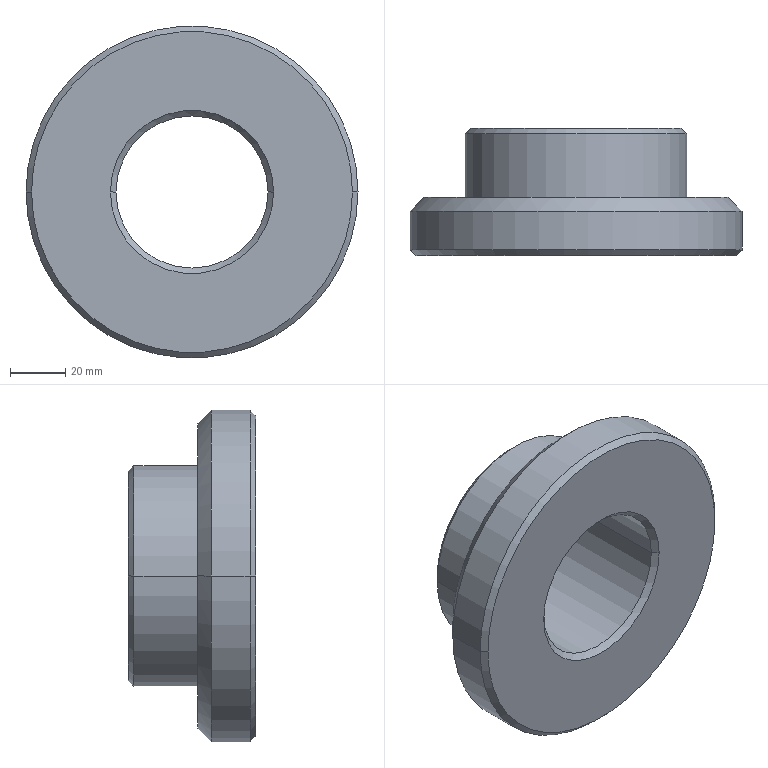Part | SolidWorks | features Revolution 1 | 1 solid | 19 faces | box 120 x 46 x 120 mm | volume 247351 mm3 | cone 10 | cylinder 6 | plane 3 | commonest cylinder face diameters 55 x2 80 x2 120 x2
STEP:
#1=CARTESIAN_POINT('',(-55.,21.,0.));
#2=VERTEX_POINT('',#1);
#3=CARTESIAN_POINT('',(55.,21.,0.));
#4=VERTEX_POINT('',#3);
#5=CARTESIAN_POINT('',(0.,21.,0.));
#6=DIRECTION('',(0.,1.,0.));
#7=DIRECTION('',(-1.,0.,0.));
#8=AXIS2_PLACEMENT_3D('',#5,#6,#7);
#9=CIRCLE('',#8,55.);
#10=EDGE_CURVE('',#2,#4,#9,.T.);
#11=ORIENTED_EDGE('',*,*,#10,.F.);
#12=CARTESIAN_POINT('',(-60.,16.,0.));
#13=VERTEX_POINT('',#12);
#14=CARTESIAN_POINT('',(-55.,21.,0.));
#15=DIRECTION('',(-0.7071,-0.7071,0.));
#16=VECTOR('',#15,1000.);
#17=LINE('',#14,#16);
#18=EDGE_CURVE('',#2,#13,#17,.T.);
#19=ORIENTED_EDGE('',*,*,#18,.T.);
#20=CARTESIAN_POINT('',(60.,16.,0.));
#21=VERTEX_POINT('',#20);
#22=CARTESIAN_POINT('',(0.,16.,0.));
#23=DIRECTION('',(0.,1.,0.));
#24=DIRECTION('',(-1.,0.,0.));
#25=AXIS2_PLACEMENT_3D('',#22,#23,#24);
#26=CIRCLE('',#25,60.);
#27=EDGE_CURVE('',#13,#21,#26,.T.);
#28=ORIENTED_EDGE('',*,*,#27,.T.);
#29=CARTESIAN_POINT('',(55.,21.,0.));
#30=DIRECTION('',(0.7071,-0.7071,0.));
#31=VECTOR('',#30,1000.);
#32=LINE('',#29,#31);
#33=EDGE_CURVE('',#4,#21,#32,.T.);
#34=ORIENTED_EDGE('',*,*,#33,.F.);
#35=EDGE_LOOP('',(#11,#19,#28,#34));
#36=FACE_OUTER_BOUND('',#35,.T.);
#37=CARTESIAN_POINT('',(0.,21.,0.));
#38=DIRECTION('',(0.,-1.,0.));
#39=DIRECTION('',(1.,0.,0.));
#40=AXIS2_PLACEMENT_3D('',#37,#38,#39);
#41=CONICAL_SURFACE('',#40,55.,0.7854);
#42=ADVANCED_FACE('',(#36),#41,.T.);
#43=CARTESIAN_POINT('',(-60.,2.,0.));
#44=VERTEX_POINT('',#43);
#45=CARTESIAN_POINT('',(60.,2.,0.));
#46=VERTEX_POINT('',#45);
#47=CARTESIAN_POINT('',(0.,2.,0.));
#48=DIRECTION('',(0.,1.,0.));
#49=DIRECTION('',(-1.,0.,0.));
#50=AXIS2_PLACEMENT_3D('',#47,#48,#49);
#51=CIRCLE('',#50,60.);
#52=EDGE_CURVE('',#44,#46,#51,.T.);
#53=ORIENTED_EDGE('',*,*,#52,.T.);
#54=CARTESIAN_POINT('',(60.,46.,0.));
#55=DIRECTION('',(0.,1.,0.));
#56=VECTOR('',#55,1000.);
#57=LINE('',#54,#56);
#58=EDGE_CURVE('',#46,#21,#57,.T.);
#59=ORIENTED_EDGE('',*,*,#58,.T.);
#60=ORIENTED_EDGE('',*,*,#27,.F.);
#61=CARTESIAN_POINT('',(-60.,46.,0.));
#62=DIRECTION('',(0.,1.,0.));
#63=VECTOR('',#62,1000.);
#64=LINE('',#61,#63);
#65=EDGE_CURVE('',#44,#13,#64,.T.);
#66=ORIENTED_EDGE('',*,*,#65,.F.);
#67=EDGE_LOOP('',(#53,#59,#60,#66));
#68=FACE_OUTER_BOUND('',#67,.T.);
#69=CARTESIAN_POINT('',(0.,46.,0.));
#70=DIRECTION('',(0.,1.,0.));
#71=DIRECTION('',(-1.,0.,0.));
#72=AXIS2_PLACEMENT_3D('',#69,#70,#71);
#73=CYLINDRICAL_SURFACE('',#72,60.);
#74=ADVANCED_FACE('',(#68),#73,.T.);
#75=CARTESIAN_POINT('',(-58.,0.,0.));
#76=VERTEX_POINT('',#75);
#77=CARTESIAN_POINT('',(58.,0.,0.));
#78=VERTEX_POINT('',#77);
#79=CARTESIAN_POINT('',(0.,0.,0.));
#80=DIRECTION('',(0.,1.,0.));
#81=DIRECTION('',(-1.,0.,0.));
#82=AXIS2_PLACEMENT_3D('',#79,#80,#81);
#83=CIRCLE('',#82,58.);
#84=EDGE_CURVE('',#76,#78,#83,.T.);
#85=ORIENTED_EDGE('',*,*,#84,.T.);
#86=CARTESIAN_POINT('',(60.,2.,0.));
#87=DIRECTION('',(0.7071,0.7071,0.));
#88=VECTOR('',#87,1000.);
#89=LINE('',#86,#88);
#90=EDGE_CURVE('',#78,#46,#89,.T.);
#91=ORIENTED_EDGE('',*,*,#90,.T.);
#92=ORIENTED_EDGE('',*,*,#52,.F.);
#93=CARTESIAN_POINT('',(-60.,2.,0.));
#94=DIRECTION('',(-0.7071,0.7071,0.));
#95=VECTOR('',#94,1000.);
#96=LINE('',#93,#95);
#97=EDGE_CURVE('',#76,#44,#96,.T.);
#98=ORIENTED_EDGE('',*,*,#97,.F.);
#99=EDGE_LOOP('',(#85,#91,#92,#98));
#100=FACE_OUTER_BOUND('',#99,.T.);
#101=CARTESIAN_POINT('',(0.,2.,0.));
#102=DIRECTION('',(0.,1.,0.));
#103=DIRECTION('',(-1.,0.,0.));
#104=AXIS2_PLACEMENT_3D('',#101,#102,#103);
#105=CONICAL_SURFACE('',#104,60.,0.7854);
#106=ADVANCED_FACE('',(#100),#105,.T.);
#107=CARTESIAN_POINT('',(27.5,2.,0.));
#108=VERTEX_POINT('',#107);
#109=CARTESIAN_POINT('',(-27.5,2.,0.));
#110=VERTEX_POINT('',#109);
#111=CARTESIAN_POINT('',(0.,2.,0.));
#112=DIRECTION('',(0.,1.,0.));
#113=DIRECTION('',(-1.,0.,0.));
#114=AXIS2_PLACEMENT_3D('',#111,#112,#113);
#115=CIRCLE('',#114,27.5);
#116=EDGE_CURVE('',#108,#110,#115,.T.);
#117=ORIENTED_EDGE('',*,*,#116,.T.);
#118=CARTESIAN_POINT('',(-29.5,0.,0.));
#119=VERTEX_POINT('',#118);
#120=CARTESIAN_POINT('',(-29.5,0.,0.));
#121=DIRECTION('',(-0.7071,-0.7071,0.));
#122=VECTOR('',#121,1000.);
#123=LINE('',#120,#122);
#124=EDGE_CURVE('',#110,#119,#123,.T.);
#125=ORIENTED_EDGE('',*,*,#124,.T.);
#126=CARTESIAN_POINT('',(29.5,0.,0.));
#127=VERTEX_POINT('',#126);
#128=CARTESIAN_POINT('',(0.,0.,0.));
#129=DIRECTION('',(0.,1.,0.));
#130=DIRECTION('',(-1.,0.,0.));
#131=AXIS2_PLACEMENT_3D('',#128,#129,#130);
#132=CIRCLE('',#131,29.5);
#133=EDGE_CURVE('',#127,#119,#132,.T.);
#134=ORIENTED_EDGE('',*,*,#133,.F.);
#135=CARTESIAN_POINT('',(29.5,0.,0.));
#136=DIRECTION('',(0.7071,-0.7071,0.));
#137=VECTOR('',#136,1000.);
#138=LINE('',#135,#137);
#139=EDGE_CURVE('',#108,#127,#138,.T.);
#140=ORIENTED_EDGE('',*,*,#139,.F.);
#141=EDGE_LOOP('',(#117,#125,#134,#140));
#142=FACE_OUTER_BOUND('',#141,.T.);
#143=CARTESIAN_POINT('',(0.,0.,0.));
#144=DIRECTION('',(0.,-1.,0.));
#145=DIRECTION('',(1.,0.,0.));
#146=AXIS2_PLACEMENT_3D('',#143,#144,#145);
#147=CONICAL_SURFACE('',#146,29.5,0.7854);
#148=ADVANCED_FACE('',(#142),#147,.F.);
#149=ORIENTED_EDGE('',*,*,#116,.F.);
#150=CARTESIAN_POINT('',(27.5,44.,0.));
#151=VERTEX_POINT('',#150);
#152=CARTESIAN_POINT('',(27.5,46.,0.));
#153=DIRECTION('',(0.,1.,0.));
#154=VECTOR('',#153,1000.);
#155=LINE('',#152,#154);
#156=EDGE_CURVE('',#108,#151,#155,.T.);
#157=ORIENTED_EDGE('',*,*,#156,.T.);
#158=CARTESIAN_POINT('',(-27.5,44.,0.));
#159=VERTEX_POINT('',#158);
#160=CARTESIAN_POINT('',(0.,44.,0.));
#161=DIRECTION('',(0.,1.,0.));
#162=DIRECTION('',(-1.,0.,0.));
#163=AXIS2_PLACEMENT_3D('',#160,#161,#162);
#164=CIRCLE('',#163,27.5);
#165=EDGE_CURVE('',#151,#159,#164,.T.);
#166=ORIENTED_EDGE('',*,*,#165,.T.);
#167=CARTESIAN_POINT('',(-27.5,46.,0.));
#168=DIRECTION('',(0.,1.,0.));
#169=VECTOR('',#168,1000.);
#170=LINE('',#167,#169);
#171=EDGE_CURVE('',#110,#159,#170,.T.);
#172=ORIENTED_EDGE('',*,*,#171,.F.);
#173=EDGE_LOOP('',(#149,#157,#166,#172));
#174=FACE_OUTER_BOUND('',#173,.T.);
#175=CARTESIAN_POINT('',(0.,46.,0.));
#176=DIRECTION('',(0.,1.,0.));
#177=DIRECTION('',(-1.,0.,0.));
#178=AXIS2_PLACEMENT_3D('',#175,#176,#177);
#179=CYLINDRICAL_SURFACE('',#178,27.5);
#180=ADVANCED_FACE('',(#174),#179,.F.);
#181=ORIENTED_EDGE('',*,*,#165,.F.);
#182=CARTESIAN_POINT('',(29.5,46.,0.));
#183=VERTEX_POINT('',#182);
#184=CARTESIAN_POINT('',(27.5,44.,0.));
#185=DIRECTION('',(0.7071,0.7071,0.));
#186=VECTOR('',#185,1000.);
#187=LINE('',#184,#186);
#188=EDGE_CURVE('',#151,#183,#187,.T.);
#189=ORIENTED_EDGE('',*,*,#188,.T.);
#190=CARTESIAN_POINT('',(-29.5,46.,0.));
#191=VERTEX_POINT('',#190);
#192=CARTESIAN_POINT('',(0.,46.,0.));
#193=DIRECTION('',(0.,1.,0.));
#194=DIRECTION('',(-1.,0.,0.));
#195=AXIS2_PLACEMENT_3D('',#192,#193,#194);
#196=CIRCLE('',#195,29.5);
#197=EDGE_CURVE('',#183,#191,#196,.T.);
#198=ORIENTED_EDGE('',*,*,#197,.T.);
#199=CARTESIAN_POINT('',(-27.5,44.,0.));
#200=DIRECTION('',(-0.7071,0.7071,0.));
#201=VECTOR('',#200,1000.);
#202=LINE('',#199,#201);
#203=EDGE_CURVE('',#159,#191,#202,.T.);
#204=ORIENTED_EDGE('',*,*,#203,.F.);
#205=EDGE_LOOP('',(#181,#189,#198,#204));
#206=FACE_OUTER_BOUND('',#205,.T.);
#207=CARTESIAN_POINT('',(0.,44.,0.));
#208=DIRECTION('',(0.,1.,0.));
#209=DIRECTION('',(-1.,0.,0.));
#210=AXIS2_PLACEMENT_3D('',#207,#208,#209);
#211=CONICAL_SURFACE('',#210,27.5,0.7854);
#212=ADVANCED_FACE('',(#206),#211,.F.);
#213=CARTESIAN_POINT('',(-38.,46.,0.));
#214=VERTEX_POINT('',#213);
#215=CARTESIAN_POINT('',(38.,46.,0.));
#216=VERTEX_POINT('',#215);
#217=CARTESIAN_POINT('',(0.,46.,0.));
#218=DIRECTION('',(0.,1.,0.));
#219=DIRECTION('',(-1.,0.,0.));
#220=AXIS2_PLACEMENT_3D('',#217,#218,#219);
#221=CIRCLE('',#220,38.);
#222=EDGE_CURVE('',#214,#216,#221,.T.);
#223=ORIENTED_EDGE('',*,*,#222,.F.);
#224=CARTESIAN_POINT('',(-40.,44.,0.));
#225=VERTEX_POINT('',#224);
#226=CARTESIAN_POINT('',(-38.,46.,0.));
#227=DIRECTION('',(-0.7071,-0.7071,0.));
#228=VECTOR('',#227,1000.);
#229=LINE('',#226,#228);
#230=EDGE_CURVE('',#214,#225,#229,.T.);
#231=ORIENTED_EDGE('',*,*,#230,.T.);
#232=CARTESIAN_POINT('',(40.,44.,0.));
#233=VERTEX_POINT('',#232);
#234=CARTESIAN_POINT('',(0.,44.,0.));
#235=DIRECTION('',(0.,1.,0.));
#236=DIRECTION('',(-1.,0.,0.));
#237=AXIS2_PLACEMENT_3D('',#234,#235,#236);
#238=CIRCLE('',#237,40.);
#239=EDGE_CURVE('',#225,#233,#238,.T.);
#240=ORIENTED_EDGE('',*,*,#239,.T.);
#241=CARTESIAN_POINT('',(38.,46.,0.));
#242=DIRECTION('',(0.7071,-0.7071,0.));
#243=VECTOR('',#242,1000.);
#244=LINE('',#241,#243);
#245=EDGE_CURVE('',#216,#233,#244,.T.);
#246=ORIENTED_EDGE('',*,*,#245,.F.);
#247=EDGE_LOOP('',(#223,#231,#240,#246));
#248=FACE_OUTER_BOUND('',#247,.T.);
#249=CARTESIAN_POINT('',(0.,46.,0.));
#250=DIRECTION('',(0.,-1.,0.));
#251=DIRECTION('',(1.,0.,0.));
#252=AXIS2_PLACEMENT_3D('',#249,#250,#251);
#253=CONICAL_SURFACE('',#252,38.,0.7854);
#254=ADVANCED_FACE('',(#248),#253,.T.);
#255=CARTESIAN_POINT('',(-40.,21.,0.));
#256=VERTEX_POINT('',#255);
#257=CARTESIAN_POINT('',(40.,21.,0.));
#258=VERTEX_POINT('',#257);
#259=CARTESIAN_POINT('',(0.,21.,0.));
#260=DIRECTION('',(0.,1.,0.));
#261=DIRECTION('',(-1.,0.,0.));
#262=AXIS2_PLACEMENT_3D('',#259,#260,#261);
#263=CIRCLE('',#262,40.);
#264=EDGE_CURVE('',#256,#258,#263,.T.);
#265=ORIENTED_EDGE('',*,*,#264,.T.);
#266=CARTESIAN_POINT('',(40.,46.,0.));
#267=DIRECTION('',(0.,1.,0.));
#268=VECTOR('',#267,1000.);
#269=LINE('',#266,#268);
#270=EDGE_CURVE('',#258,#233,#269,.T.);
#271=ORIENTED_EDGE('',*,*,#270,.T.);
#272=ORIENTED_EDGE('',*,*,#239,.F.);
#273=CARTESIAN_POINT('',(-40.,46.,0.));
#274=DIRECTION('',(0.,1.,0.));
#275=VECTOR('',#274,1000.);
#276=LINE('',#273,#275);
#277=EDGE_CURVE('',#256,#225,#276,.T.);
#278=ORIENTED_EDGE('',*,*,#277,.F.);
#279=EDGE_LOOP('',(#265,#271,#272,#278));
#280=FACE_OUTER_BOUND('',#279,.T.);
#281=CARTESIAN_POINT('',(0.,46.,0.));
#282=DIRECTION('',(0.,1.,0.));
#283=DIRECTION('',(-1.,0.,0.));
#284=AXIS2_PLACEMENT_3D('',#281,#282,#283);
#285=CYLINDRICAL_SURFACE('',#284,40.);
#286=ADVANCED_FACE('',(#280),#285,.T.);
#287=ORIENTED_EDGE('',*,*,#270,.F.);
#288=CARTESIAN_POINT('',(0.,21.,0.));
#289=DIRECTION('',(0.,1.,0.));
#290=DIRECTION('',(-1.,0.,0.));
#291=AXIS2_PLACEMENT_3D('',#288,#289,#290);
#292=CIRCLE('',#291,40.);
#293=EDGE_CURVE('',#258,#256,#292,.T.);
#294=ORIENTED_EDGE('',*,*,#293,.T.);
#295=ORIENTED_EDGE('',*,*,#277,.T.);
#296=CARTESIAN_POINT('',(0.,44.,0.));
#297=DIRECTION('',(0.,1.,0.));
#298=DIRECTION('',(-1.,0.,0.));
#299=AXIS2_PLACEMENT_3D('',#296,#297,#298);
#300=CIRCLE('',#299,40.);
#301=EDGE_CURVE('',#233,#225,#300,.T.);
#302=ORIENTED_EDGE('',*,*,#301,.F.);
#303=EDGE_LOOP('',(#287,#294,#295,#302));
#304=FACE_OUTER_BOUND('',#303,.T.);
#305=CARTESIAN_POINT('',(0.,46.,0.));
#306=DIRECTION('',(0.,1.,0.));
#307=DIRECTION('',(-1.,0.,0.));
#308=AXIS2_PLACEMENT_3D('',#305,#306,#307);
#309=CYLINDRICAL_SURFACE('',#308,40.);
#310=ADVANCED_FACE('',(#304),#309,.T.);
#311=ORIENTED_EDGE('',*,*,#230,.F.);
#312=CARTESIAN_POINT('',(0.,46.,0.));
#313=DIRECTION('',(0.,1.,0.));
#314=DIRECTION('',(-1.,0.,0.));
#315=AXIS2_PLACEMENT_3D('',#312,#313,#314);
#316=CIRCLE('',#315,38.);
#317=EDGE_CURVE('',#216,#214,#316,.T.);
#318=ORIENTED_EDGE('',*,*,#317,.F.);
#319=ORIENTED_EDGE('',*,*,#245,.T.);
#320=ORIENTED_EDGE('',*,*,#301,.T.);
#321=EDGE_LOOP('',(#311,#318,#319,#320));
#322=FACE_OUTER_BOUND('',#321,.T.);
#323=CARTESIAN_POINT('',(0.,46.,0.));
#324=DIRECTION('',(0.,-1.,0.));
#325=DIRECTION('',(1.,0.,0.));
#326=AXIS2_PLACEMENT_3D('',#323,#324,#325);
#327=CONICAL_SURFACE('',#326,38.,0.7854);
#328=ADVANCED_FACE('',(#322),#327,.T.);
#329=ORIENTED_EDGE('',*,*,#317,.T.);
#330=ORIENTED_EDGE('',*,*,#222,.T.);
#331=EDGE_LOOP('',(#329,#330));
#332=FACE_OUTER_BOUND('',#331,.T.);
#333=CARTESIAN_POINT('',(0.,46.,0.));
#334=DIRECTION('',(0.,1.,0.));
#335=DIRECTION('',(-1.,0.,0.));
#336=AXIS2_PLACEMENT_3D('',#333,#334,#335);
#337=CIRCLE('',#336,29.5);
#338=EDGE_CURVE('',#191,#183,#337,.T.);
#339=ORIENTED_EDGE('',*,*,#338,.F.);
#340=ORIENTED_EDGE('',*,*,#197,.F.);
#341=EDGE_LOOP('',(#339,#340));
#342=FACE_BOUND('',#341,.T.);
#343=CARTESIAN_POINT('',(-38.,46.,0.));
#344=DIRECTION('',(0.,1.,0.));
#345=DIRECTION('',(-1.,0.,0.));
#346=AXIS2_PLACEMENT_3D('',#343,#344,#345);
#347=PLANE('',#346);
#348=ADVANCED_FACE('',(#332,#342),#347,.T.);
#349=ORIENTED_EDGE('',*,*,#188,.F.);
#350=CARTESIAN_POINT('',(0.,44.,0.));
#351=DIRECTION('',(0.,1.,0.));
#352=DIRECTION('',(-1.,0.,0.));
#353=AXIS2_PLACEMENT_3D('',#350,#351,#352);
#354=CIRCLE('',#353,27.5);
#355=EDGE_CURVE('',#159,#151,#354,.T.);
#356=ORIENTED_EDGE('',*,*,#355,.F.);
#357=ORIENTED_EDGE('',*,*,#203,.T.);
#358=ORIENTED_EDGE('',*,*,#338,.T.);
#359=EDGE_LOOP('',(#349,#356,#357,#358));
#360=FACE_OUTER_BOUND('',#359,.T.);
#361=CARTESIAN_POINT('',(0.,44.,0.));
#362=DIRECTION('',(0.,1.,0.));
#363=DIRECTION('',(-1.,0.,0.));
#364=AXIS2_PLACEMENT_3D('',#361,#362,#363);
#365=CONICAL_SURFACE('',#364,27.5,0.7854);
#366=ADVANCED_FACE('',(#360),#365,.F.);
#367=ORIENTED_EDGE('',*,*,#156,.F.);
#368=CARTESIAN_POINT('',(0.,2.,0.));
#369=DIRECTION('',(0.,1.,0.));
#370=DIRECTION('',(-1.,0.,0.));
#371=AXIS2_PLACEMENT_3D('',#368,#369,#370);
#372=CIRCLE('',#371,27.5);
#373=EDGE_CURVE('',#110,#108,#372,.T.);
#374=ORIENTED_EDGE('',*,*,#373,.F.);
#375=ORIENTED_EDGE('',*,*,#171,.T.);
#376=ORIENTED_EDGE('',*,*,#355,.T.);
#377=EDGE_LOOP('',(#367,#374,#375,#376));
#378=FACE_OUTER_BOUND('',#377,.T.);
#379=CARTESIAN_POINT('',(0.,46.,0.));
#380=DIRECTION('',(0.,1.,0.));
#381=DIRECTION('',(-1.,0.,0.));
#382=AXIS2_PLACEMENT_3D('',#379,#380,#381);
#383=CYLINDRICAL_SURFACE('',#382,27.5);
#384=ADVANCED_FACE('',(#378),#383,.F.);
#385=ORIENTED_EDGE('',*,*,#124,.F.);
#386=ORIENTED_EDGE('',*,*,#373,.T.);
#387=ORIENTED_EDGE('',*,*,#139,.T.);
#388=CARTESIAN_POINT('',(0.,0.,0.));
#389=DIRECTION('',(0.,1.,0.));
#390=DIRECTION('',(-1.,0.,0.));
#391=AXIS2_PLACEMENT_3D('',#388,#389,#390);
#392=CIRCLE('',#391,29.5);
#393=EDGE_CURVE('',#119,#127,#392,.T.);
#394=ORIENTED_EDGE('',*,*,#393,.F.);
#395=EDGE_LOOP('',(#385,#386,#387,#394));
#396=FACE_OUTER_BOUND('',#395,.T.);
#397=CARTESIAN_POINT('',(0.,0.,0.));
#398=DIRECTION('',(0.,-1.,0.));
#399=DIRECTION('',(1.,0.,0.));
#400=AXIS2_PLACEMENT_3D('',#397,#398,#399);
#401=CONICAL_SURFACE('',#400,29.5,0.7854);
#402=ADVANCED_FACE('',(#396),#401,.F.);
#403=ORIENTED_EDGE('',*,*,#133,.T.);
#404=ORIENTED_EDGE('',*,*,#393,.T.);
#405=EDGE_LOOP('',(#403,#404));
#406=FACE_BOUND('',#405,.T.);
#407=ORIENTED_EDGE('',*,*,#84,.F.);
#408=CARTESIAN_POINT('',(0.,0.,0.));
#409=DIRECTION('',(0.,1.,0.));
#410=DIRECTION('',(-1.,0.,0.));
#411=AXIS2_PLACEMENT_3D('',#408,#409,#410);
#412=CIRCLE('',#411,58.);
#413=EDGE_CURVE('',#78,#76,#412,.T.);
#414=ORIENTED_EDGE('',*,*,#413,.F.);
#415=EDGE_LOOP('',(#407,#414));
#416=FACE_OUTER_BOUND('',#415,.T.);
#417=CARTESIAN_POINT('',(-29.5,0.,0.));
#418=DIRECTION('',(0.,-1.,0.));
#419=DIRECTION('',(1.,0.,0.));
#420=AXIS2_PLACEMENT_3D('',#417,#418,#419);
#421=PLANE('',#420);
#422=ADVANCED_FACE('',(#406,#416),#421,.T.);
#423=ORIENTED_EDGE('',*,*,#90,.F.);
#424=ORIENTED_EDGE('',*,*,#413,.T.);
#425=ORIENTED_EDGE('',*,*,#97,.T.);
#426=CARTESIAN_POINT('',(0.,2.,0.));
#427=DIRECTION('',(0.,1.,0.));
#428=DIRECTION('',(-1.,0.,0.));
#429=AXIS2_PLACEMENT_3D('',#426,#427,#428);
#430=CIRCLE('',#429,60.);
#431=EDGE_CURVE('',#46,#44,#430,.T.);
#432=ORIENTED_EDGE('',*,*,#431,.F.);
#433=EDGE_LOOP('',(#423,#424,#425,#432));
#434=FACE_OUTER_BOUND('',#433,.T.);
#435=CARTESIAN_POINT('',(0.,2.,0.));
#436=DIRECTION('',(0.,1.,0.));
#437=DIRECTION('',(-1.,0.,0.));
#438=AXIS2_PLACEMENT_3D('',#435,#436,#437);
#439=CONICAL_SURFACE('',#438,60.,0.7854);
#440=ADVANCED_FACE('',(#434),#439,.T.);
#441=ORIENTED_EDGE('',*,*,#58,.F.);
#442=ORIENTED_EDGE('',*,*,#431,.T.);
#443=ORIENTED_EDGE('',*,*,#65,.T.);
#444=CARTESIAN_POINT('',(0.,16.,0.));
#445=DIRECTION('',(0.,1.,0.));
#446=DIRECTION('',(-1.,0.,0.));
#447=AXIS2_PLACEMENT_3D('',#444,#445,#446);
#448=CIRCLE('',#447,60.);
#449=EDGE_CURVE('',#21,#13,#448,.T.);
#450=ORIENTED_EDGE('',*,*,#449,.F.);
#451=EDGE_LOOP('',(#441,#442,#443,#450));
#452=FACE_OUTER_BOUND('',#451,.T.);
#453=CARTESIAN_POINT('',(0.,46.,0.));
#454=DIRECTION('',(0.,1.,0.));
#455=DIRECTION('',(-1.,0.,0.));
#456=AXIS2_PLACEMENT_3D('',#453,#454,#455);
#457=CYLINDRICAL_SURFACE('',#456,60.);
#458=ADVANCED_FACE('',(#452),#457,.T.);
#459=ORIENTED_EDGE('',*,*,#18,.F.);
#460=CARTESIAN_POINT('',(0.,21.,0.));
#461=DIRECTION('',(0.,1.,0.));
#462=DIRECTION('',(-1.,0.,0.));
#463=AXIS2_PLACEMENT_3D('',#460,#461,#462);
#464=CIRCLE('',#463,55.);
#465=EDGE_CURVE('',#4,#2,#464,.T.);
#466=ORIENTED_EDGE('',*,*,#465,.F.);
#467=ORIENTED_EDGE('',*,*,#33,.T.);
#468=ORIENTED_EDGE('',*,*,#449,.T.);
#469=EDGE_LOOP('',(#459,#466,#467,#468));
#470=FACE_OUTER_BOUND('',#469,.T.);
#471=CARTESIAN_POINT('',(0.,21.,0.));
#472=DIRECTION('',(0.,-1.,0.));
#473=DIRECTION('',(1.,0.,0.));
#474=AXIS2_PLACEMENT_3D('',#471,#472,#473);
#475=CONICAL_SURFACE('',#474,55.,0.7854);
#476=ADVANCED_FACE('',(#470),#475,.T.);
#477=ORIENTED_EDGE('',*,*,#465,.T.);
#478=ORIENTED_EDGE('',*,*,#10,.T.);
#479=EDGE_LOOP('',(#477,#478));
#480=FACE_OUTER_BOUND('',#479,.T.);
#481=ORIENTED_EDGE('',*,*,#264,.F.);
#482=ORIENTED_EDGE('',*,*,#293,.F.);
#483=EDGE_LOOP('',(#481,#482));
#484=FACE_BOUND('',#483,.T.);
#485=CARTESIAN_POINT('',(-55.,21.,0.));
#486=DIRECTION('',(0.,1.,0.));
#487=DIRECTION('',(-1.,0.,0.));
#488=AXIS2_PLACEMENT_3D('',#485,#486,#487);
#489=PLANE('',#488);
#490=ADVANCED_FACE('',(#480,#484),#489,.T.);
#491=CLOSED_SHELL('',(#42,#74,#106,#148,#180,#212,#254,#286,#310,#328,#348,#366,#384,#402,#422,#440,#458,#476,#490));
#492=MANIFOLD_SOLID_BREP('',#491);
#493=CARTESIAN_POINT('',(0.,0.,0.));
#494=DIRECTION('',(0.,0.,1.));
#495=DIRECTION('',(1.,0.,0.));
#496=AXIS2_PLACEMENT_3D('',#493,#494,#495);
#497=(LENGTH_UNIT()NAMED_UNIT(*)SI_UNIT(.MILLI.,.METRE.));
#498=UNCERTAINTY_MEASURE_WITH_UNIT(LENGTH_MEASURE(0.00001),#497,'','');
#499=(NAMED_UNIT(*)PLANE_ANGLE_UNIT()SI_UNIT($,.RADIAN.));
#500=(NAMED_UNIT(*)SI_UNIT($,.STERADIAN.)SOLID_ANGLE_UNIT());
#501=(GEOMETRIC_REPRESENTATION_CONTEXT(3)GLOBAL_UNCERTAINTY_ASSIGNED_CONTEXT((#498))GLOBAL_UNIT_ASSIGNED_CONTEXT((#497,#499,#500))REPRESENTATION_CONTEXT('',''));
#502=ADVANCED_BREP_SHAPE_REPRESENTATION('',(#492,#496),#501);